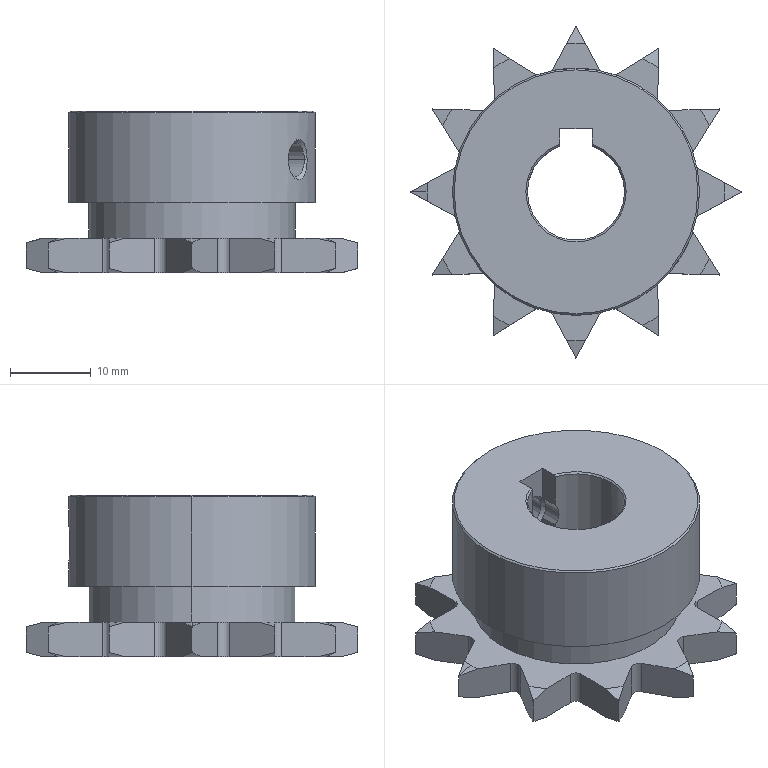Part | STEP file | SP35B12_N_12_SP35B12-N-12 | 1 solid | 135 faces | box 41 x 41 x 20 mm | volume 11740 mm3 | cone 42 | plane 34 | cylinder 33 | torus 26 | commonest cylinder face diameters 2 x16 5 x6 4.134 x4 12 x3 25.5 x2 30.5 x2